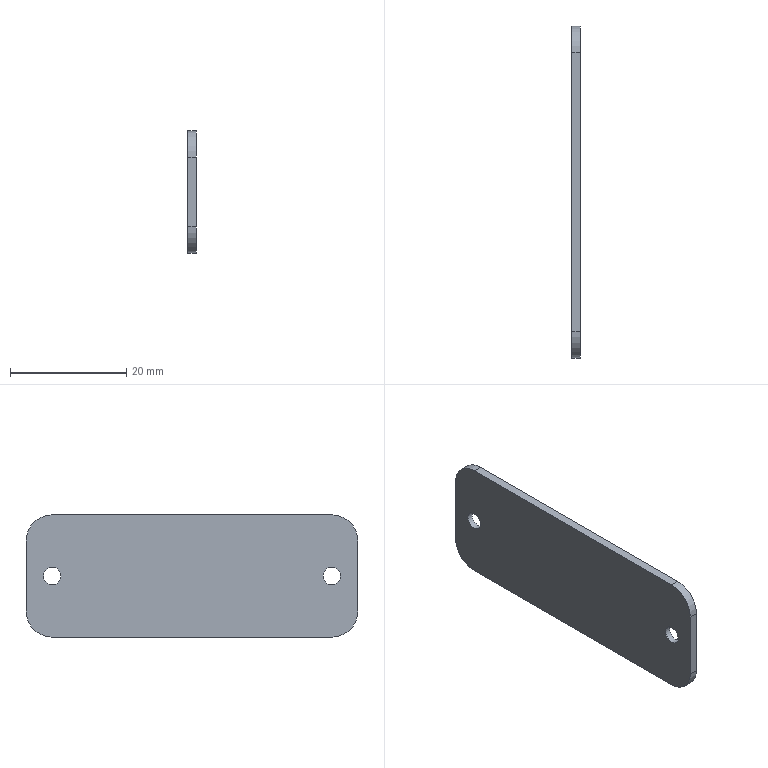Part | STEP file | 1-38 | 1 solid | 79 faces | box 1.5 x 57 x 21 mm | volume 1289 mm3 | plane 35 | spline 34 | cylinder 10 | commonest cylinder face diameters 6 x4 9 x4 3 x2